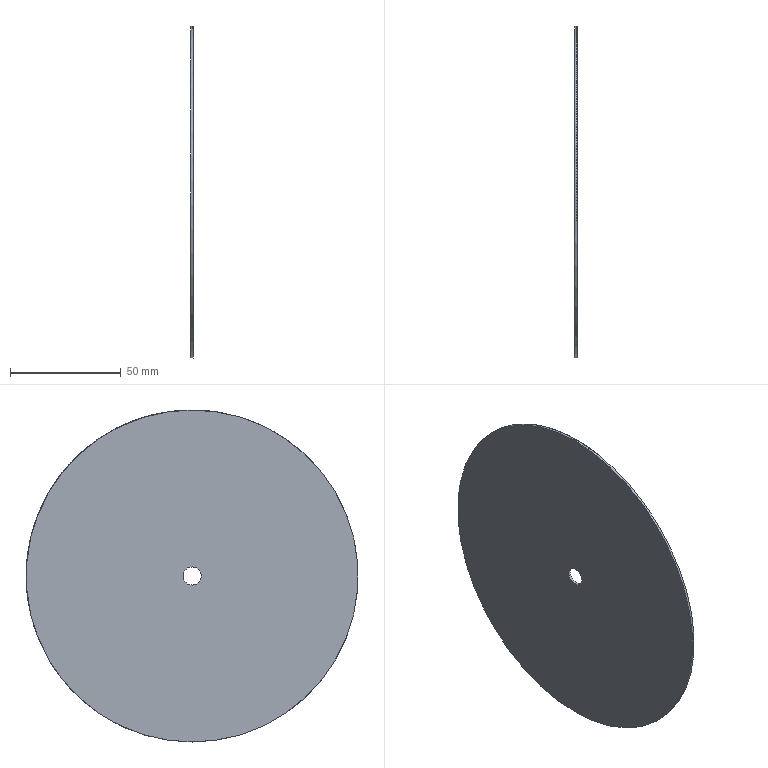Part | SolidWorks | features ICE 5, CirPattern 3, Extrusion 1 | 1 solid | 813 faces | box 1 x 150 x 150 mm | volume 17590 mm3 | plane 563 | spline 246 | cylinder 4 | commonest cylinder face diameters 8.2 x2 150 x2